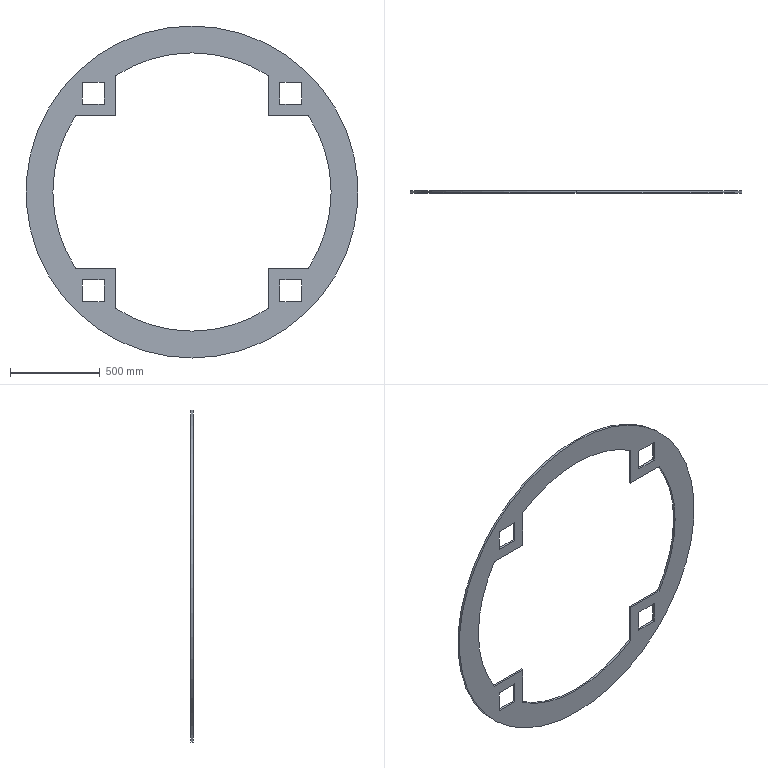Part | SolidWorks | features Extrusion 1 | 1 solid | 33 faces | box 1850 x 12 x 1850 mm | volume 10257241 mm3 | plane 26 | cylinder 7 | commonest cylinder face diameters 1550 x5 1850 x2
STEP:
#1=CARTESIAN_POINT('',(0.,12.,925.));
#2=VERTEX_POINT('',#1);
#3=CARTESIAN_POINT('',(0.,12.,-925.));
#4=VERTEX_POINT('',#3);
#5=CARTESIAN_POINT('',(0.,12.,0.));
#6=DIRECTION('',(0.,1.,0.));
#7=DIRECTION('',(0.,0.,1.));
#8=AXIS2_PLACEMENT_3D('',#5,#6,#7);
#9=CIRCLE('',#8,925.);
#10=EDGE_CURVE('',#2,#4,#9,.T.);
#11=ORIENTED_EDGE('',*,*,#10,.F.);
#12=CARTESIAN_POINT('',(0.,0.,925.));
#13=VERTEX_POINT('',#12);
#14=CARTESIAN_POINT('',(0.,12.,925.));
#15=DIRECTION('',(0.,-1.,0.));
#16=VECTOR('',#15,1000.);
#17=LINE('',#14,#16);
#18=EDGE_CURVE('',#2,#13,#17,.T.);
#19=ORIENTED_EDGE('',*,*,#18,.T.);
#20=CARTESIAN_POINT('',(0.,0.,-925.));
#21=VERTEX_POINT('',#20);
#22=CARTESIAN_POINT('',(0.,0.,0.));
#23=DIRECTION('',(0.,1.,0.));
#24=DIRECTION('',(0.,0.,1.));
#25=AXIS2_PLACEMENT_3D('',#22,#23,#24);
#26=CIRCLE('',#25,925.);
#27=EDGE_CURVE('',#13,#21,#26,.T.);
#28=ORIENTED_EDGE('',*,*,#27,.T.);
#29=CARTESIAN_POINT('',(0.,12.,-925.));
#30=DIRECTION('',(0.,-1.,0.));
#31=VECTOR('',#30,1000.);
#32=LINE('',#29,#31);
#33=EDGE_CURVE('',#4,#21,#32,.T.);
#34=ORIENTED_EDGE('',*,*,#33,.F.);
#35=EDGE_LOOP('',(#11,#19,#28,#34));
#36=FACE_OUTER_BOUND('',#35,.T.);
#37=CARTESIAN_POINT('',(0.,12.,0.));
#38=DIRECTION('',(0.,-1.,0.));
#39=DIRECTION('',(0.,0.,-1.));
#40=AXIS2_PLACEMENT_3D('',#37,#38,#39);
#41=CYLINDRICAL_SURFACE('',#40,925.);
#42=ADVANCED_FACE('',(#36),#41,.T.);
#43=CARTESIAN_POINT('',(425.,12.,-648.074));
#44=VERTEX_POINT('',#43);
#45=CARTESIAN_POINT('',(0.,12.,-775.));
#46=VERTEX_POINT('',#45);
#47=CARTESIAN_POINT('',(0.,12.,0.));
#48=DIRECTION('',(0.,1.,0.));
#49=DIRECTION('',(0.,0.,1.));
#50=AXIS2_PLACEMENT_3D('',#47,#48,#49);
#51=CIRCLE('',#50,775.);
#52=EDGE_CURVE('',#44,#46,#51,.T.);
#53=ORIENTED_EDGE('',*,*,#52,.T.);
#54=CARTESIAN_POINT('',(0.,0.,-775.));
#55=VERTEX_POINT('',#54);
#56=CARTESIAN_POINT('',(0.,12.,-775.));
#57=DIRECTION('',(0.,-1.,0.));
#58=VECTOR('',#57,1000.);
#59=LINE('',#56,#58);
#60=EDGE_CURVE('',#46,#55,#59,.T.);
#61=ORIENTED_EDGE('',*,*,#60,.T.);
#62=CARTESIAN_POINT('',(425.,0.,-648.074));
#63=VERTEX_POINT('',#62);
#64=CARTESIAN_POINT('',(0.,0.,0.));
#65=DIRECTION('',(0.,1.,0.));
#66=DIRECTION('',(0.,0.,1.));
#67=AXIS2_PLACEMENT_3D('',#64,#65,#66);
#68=CIRCLE('',#67,775.);
#69=EDGE_CURVE('',#63,#55,#68,.T.);
#70=ORIENTED_EDGE('',*,*,#69,.F.);
#71=CARTESIAN_POINT('',(425.,12.,-648.074));
#72=DIRECTION('',(0.,-1.,0.));
#73=VECTOR('',#72,1000.);
#74=LINE('',#71,#73);
#75=EDGE_CURVE('',#44,#63,#74,.T.);
#76=ORIENTED_EDGE('',*,*,#75,.F.);
#77=EDGE_LOOP('',(#53,#61,#70,#76));
#78=FACE_OUTER_BOUND('',#77,.T.);
#79=CARTESIAN_POINT('',(0.,12.,0.));
#80=DIRECTION('',(0.,-1.,0.));
#81=DIRECTION('',(0.,0.,-1.));
#82=AXIS2_PLACEMENT_3D('',#79,#80,#81);
#83=CYLINDRICAL_SURFACE('',#82,775.);
#84=ADVANCED_FACE('',(#78),#83,.F.);
#85=CARTESIAN_POINT('',(-489.,0.,-489.));
#86=VERTEX_POINT('',#85);
#87=CARTESIAN_POINT('',(-489.,0.,-611.));
#88=VERTEX_POINT('',#87);
#89=CARTESIAN_POINT('',(-489.,0.,0.));
#90=DIRECTION('',(0.,0.,-1.));
#91=VECTOR('',#90,1000.);
#92=LINE('',#89,#91);
#93=EDGE_CURVE('',#86,#88,#92,.T.);
#94=ORIENTED_EDGE('',*,*,#93,.F.);
#95=CARTESIAN_POINT('',(-489.,12.,-489.));
#96=VERTEX_POINT('',#95);
#97=CARTESIAN_POINT('',(-489.,12.,-489.));
#98=DIRECTION('',(0.,-1.,0.));
#99=VECTOR('',#98,1000.);
#100=LINE('',#97,#99);
#101=EDGE_CURVE('',#96,#86,#100,.T.);
#102=ORIENTED_EDGE('',*,*,#101,.F.);
#103=CARTESIAN_POINT('',(-489.,12.,-611.));
#104=VERTEX_POINT('',#103);
#105=CARTESIAN_POINT('',(-489.,12.,0.));
#106=DIRECTION('',(0.,0.,-1.));
#107=VECTOR('',#106,1000.);
#108=LINE('',#105,#107);
#109=EDGE_CURVE('',#96,#104,#108,.T.);
#110=ORIENTED_EDGE('',*,*,#109,.T.);
#111=CARTESIAN_POINT('',(-489.,12.,-611.));
#112=DIRECTION('',(0.,-1.,0.));
#113=VECTOR('',#112,1000.);
#114=LINE('',#111,#113);
#115=EDGE_CURVE('',#104,#88,#114,.T.);
#116=ORIENTED_EDGE('',*,*,#115,.T.);
#117=EDGE_LOOP('',(#94,#102,#110,#116));
#118=FACE_OUTER_BOUND('',#117,.T.);
#119=CARTESIAN_POINT('',(-489.,12.,0.));
#120=DIRECTION('',(-1.,0.,0.));
#121=DIRECTION('',(0.,0.,1.));
#122=AXIS2_PLACEMENT_3D('',#119,#120,#121);
#123=PLANE('',#122);
#124=ADVANCED_FACE('',(#118),#123,.T.);
#125=CARTESIAN_POINT('',(-611.,0.,-489.));
#126=VERTEX_POINT('',#125);
#127=CARTESIAN_POINT('',(0.,0.,-489.));
#128=DIRECTION('',(-1.,0.,0.));
#129=VECTOR('',#128,1000.);
#130=LINE('',#127,#129);
#131=EDGE_CURVE('',#86,#126,#130,.T.);
#132=ORIENTED_EDGE('',*,*,#131,.T.);
#133=CARTESIAN_POINT('',(-611.,12.,-489.));
#134=VERTEX_POINT('',#133);
#135=CARTESIAN_POINT('',(-611.,12.,-489.));
#136=DIRECTION('',(0.,-1.,0.));
#137=VECTOR('',#136,1000.);
#138=LINE('',#135,#137);
#139=EDGE_CURVE('',#134,#126,#138,.T.);
#140=ORIENTED_EDGE('',*,*,#139,.F.);
#141=CARTESIAN_POINT('',(0.,12.,-489.));
#142=DIRECTION('',(-1.,0.,0.));
#143=VECTOR('',#142,1000.);
#144=LINE('',#141,#143);
#145=EDGE_CURVE('',#96,#134,#144,.T.);
#146=ORIENTED_EDGE('',*,*,#145,.F.);
#147=ORIENTED_EDGE('',*,*,#101,.T.);
#148=EDGE_LOOP('',(#132,#140,#146,#147));
#149=FACE_OUTER_BOUND('',#148,.T.);
#150=CARTESIAN_POINT('',(0.,12.,-489.));
#151=DIRECTION('',(0.,0.,1.));
#152=DIRECTION('',(1.,0.,0.));
#153=AXIS2_PLACEMENT_3D('',#150,#151,#152);
#154=PLANE('',#153);
#155=ADVANCED_FACE('',(#149),#154,.F.);
#156=CARTESIAN_POINT('',(-611.,0.,-611.));
#157=VERTEX_POINT('',#156);
#158=CARTESIAN_POINT('',(-611.,0.,0.));
#159=DIRECTION('',(0.,0.,-1.));
#160=VECTOR('',#159,1000.);
#161=LINE('',#158,#160);
#162=EDGE_CURVE('',#126,#157,#161,.T.);
#163=ORIENTED_EDGE('',*,*,#162,.T.);
#164=CARTESIAN_POINT('',(-611.,12.,-611.));
#165=VERTEX_POINT('',#164);
#166=CARTESIAN_POINT('',(-611.,12.,-611.));
#167=DIRECTION('',(0.,-1.,0.));
#168=VECTOR('',#167,1000.);
#169=LINE('',#166,#168);
#170=EDGE_CURVE('',#165,#157,#169,.T.);
#171=ORIENTED_EDGE('',*,*,#170,.F.);
#172=CARTESIAN_POINT('',(-611.,12.,0.));
#173=DIRECTION('',(0.,0.,-1.));
#174=VECTOR('',#173,1000.);
#175=LINE('',#172,#174);
#176=EDGE_CURVE('',#134,#165,#175,.T.);
#177=ORIENTED_EDGE('',*,*,#176,.F.);
#178=ORIENTED_EDGE('',*,*,#139,.T.);
#179=EDGE_LOOP('',(#163,#171,#177,#178));
#180=FACE_OUTER_BOUND('',#179,.T.);
#181=CARTESIAN_POINT('',(-611.,12.,0.));
#182=DIRECTION('',(-1.,0.,0.));
#183=DIRECTION('',(0.,0.,1.));
#184=AXIS2_PLACEMENT_3D('',#181,#182,#183);
#185=PLANE('',#184);
#186=ADVANCED_FACE('',(#180),#185,.F.);
#187=CARTESIAN_POINT('',(-489.,0.,489.));
#188=VERTEX_POINT('',#187);
#189=CARTESIAN_POINT('',(-611.,0.,489.));
#190=VERTEX_POINT('',#189);
#191=CARTESIAN_POINT('',(0.,0.,489.));
#192=DIRECTION('',(-1.,0.,0.));
#193=VECTOR('',#192,1000.);
#194=LINE('',#191,#193);
#195=EDGE_CURVE('',#188,#190,#194,.T.);
#196=ORIENTED_EDGE('',*,*,#195,.F.);
#197=CARTESIAN_POINT('',(-489.,12.,489.));
#198=VERTEX_POINT('',#197);
#199=CARTESIAN_POINT('',(-489.,12.,489.));
#200=DIRECTION('',(0.,-1.,0.));
#201=VECTOR('',#200,1000.);
#202=LINE('',#199,#201);
#203=EDGE_CURVE('',#198,#188,#202,.T.);
#204=ORIENTED_EDGE('',*,*,#203,.F.);
#205=CARTESIAN_POINT('',(-611.,12.,489.));
#206=VERTEX_POINT('',#205);
#207=CARTESIAN_POINT('',(0.,12.,489.));
#208=DIRECTION('',(-1.,0.,0.));
#209=VECTOR('',#208,1000.);
#210=LINE('',#207,#209);
#211=EDGE_CURVE('',#198,#206,#210,.T.);
#212=ORIENTED_EDGE('',*,*,#211,.T.);
#213=CARTESIAN_POINT('',(-611.,12.,489.));
#214=DIRECTION('',(0.,-1.,0.));
#215=VECTOR('',#214,1000.);
#216=LINE('',#213,#215);
#217=EDGE_CURVE('',#206,#190,#216,.T.);
#218=ORIENTED_EDGE('',*,*,#217,.T.);
#219=EDGE_LOOP('',(#196,#204,#212,#218));
#220=FACE_OUTER_BOUND('',#219,.T.);
#221=CARTESIAN_POINT('',(0.,12.,489.));
#222=DIRECTION('',(0.,0.,1.));
#223=DIRECTION('',(1.,0.,0.));
#224=AXIS2_PLACEMENT_3D('',#221,#222,#223);
#225=PLANE('',#224);
#226=ADVANCED_FACE('',(#220),#225,.T.);
#227=CARTESIAN_POINT('',(-489.,0.,611.));
#228=VERTEX_POINT('',#227);
#229=CARTESIAN_POINT('',(-489.,0.,0.));
#230=DIRECTION('',(0.,0.,1.));
#231=VECTOR('',#230,1000.);
#232=LINE('',#229,#231);
#233=EDGE_CURVE('',#188,#228,#232,.T.);
#234=ORIENTED_EDGE('',*,*,#233,.T.);
#235=CARTESIAN_POINT('',(-489.,12.,611.));
#236=VERTEX_POINT('',#235);
#237=CARTESIAN_POINT('',(-489.,12.,611.));
#238=DIRECTION('',(0.,-1.,0.));
#239=VECTOR('',#238,1000.);
#240=LINE('',#237,#239);
#241=EDGE_CURVE('',#236,#228,#240,.T.);
#242=ORIENTED_EDGE('',*,*,#241,.F.);
#243=CARTESIAN_POINT('',(-489.,12.,0.));
#244=DIRECTION('',(0.,0.,1.));
#245=VECTOR('',#244,1000.);
#246=LINE('',#243,#245);
#247=EDGE_CURVE('',#198,#236,#246,.T.);
#248=ORIENTED_EDGE('',*,*,#247,.F.);
#249=ORIENTED_EDGE('',*,*,#203,.T.);
#250=EDGE_LOOP('',(#234,#242,#248,#249));
#251=FACE_OUTER_BOUND('',#250,.T.);
#252=CARTESIAN_POINT('',(-489.,12.,0.));
#253=DIRECTION('',(1.,0.,0.));
#254=DIRECTION('',(0.,0.,-1.));
#255=AXIS2_PLACEMENT_3D('',#252,#253,#254);
#256=PLANE('',#255);
#257=ADVANCED_FACE('',(#251),#256,.F.);
#258=CARTESIAN_POINT('',(-611.,0.,611.));
#259=VERTEX_POINT('',#258);
#260=CARTESIAN_POINT('',(0.,0.,611.));
#261=DIRECTION('',(-1.,0.,0.));
#262=VECTOR('',#261,1000.);
#263=LINE('',#260,#262);
#264=EDGE_CURVE('',#228,#259,#263,.T.);
#265=ORIENTED_EDGE('',*,*,#264,.T.);
#266=CARTESIAN_POINT('',(-611.,12.,611.));
#267=VERTEX_POINT('',#266);
#268=CARTESIAN_POINT('',(-611.,12.,611.));
#269=DIRECTION('',(0.,-1.,0.));
#270=VECTOR('',#269,1000.);
#271=LINE('',#268,#270);
#272=EDGE_CURVE('',#267,#259,#271,.T.);
#273=ORIENTED_EDGE('',*,*,#272,.F.);
#274=CARTESIAN_POINT('',(0.,12.,611.));
#275=DIRECTION('',(-1.,0.,0.));
#276=VECTOR('',#275,1000.);
#277=LINE('',#274,#276);
#278=EDGE_CURVE('',#236,#267,#277,.T.);
#279=ORIENTED_EDGE('',*,*,#278,.F.);
#280=ORIENTED_EDGE('',*,*,#241,.T.);
#281=EDGE_LOOP('',(#265,#273,#279,#280));
#282=FACE_OUTER_BOUND('',#281,.T.);
#283=CARTESIAN_POINT('',(0.,12.,611.));
#284=DIRECTION('',(0.,0.,1.));
#285=DIRECTION('',(1.,0.,0.));
#286=AXIS2_PLACEMENT_3D('',#283,#284,#285);
#287=PLANE('',#286);
#288=ADVANCED_FACE('',(#282),#287,.F.);
#289=CARTESIAN_POINT('',(489.,0.,489.));
#290=VERTEX_POINT('',#289);
#291=CARTESIAN_POINT('',(489.,0.,611.));
#292=VERTEX_POINT('',#291);
#293=CARTESIAN_POINT('',(489.,0.,0.));
#294=DIRECTION('',(0.,0.,1.));
#295=VECTOR('',#294,1000.);
#296=LINE('',#293,#295);
#297=EDGE_CURVE('',#290,#292,#296,.T.);
#298=ORIENTED_EDGE('',*,*,#297,.F.);
#299=CARTESIAN_POINT('',(489.,12.,489.));
#300=VERTEX_POINT('',#299);
#301=CARTESIAN_POINT('',(489.,12.,489.));
#302=DIRECTION('',(0.,-1.,0.));
#303=VECTOR('',#302,1000.);
#304=LINE('',#301,#303);
#305=EDGE_CURVE('',#300,#290,#304,.T.);
#306=ORIENTED_EDGE('',*,*,#305,.F.);
#307=CARTESIAN_POINT('',(489.,12.,611.));
#308=VERTEX_POINT('',#307);
#309=CARTESIAN_POINT('',(489.,12.,0.));
#310=DIRECTION('',(0.,0.,1.));
#311=VECTOR('',#310,1000.);
#312=LINE('',#309,#311);
#313=EDGE_CURVE('',#300,#308,#312,.T.);
#314=ORIENTED_EDGE('',*,*,#313,.T.);
#315=CARTESIAN_POINT('',(489.,12.,611.));
#316=DIRECTION('',(0.,-1.,0.));
#317=VECTOR('',#316,1000.);
#318=LINE('',#315,#317);
#319=EDGE_CURVE('',#308,#292,#318,.T.);
#320=ORIENTED_EDGE('',*,*,#319,.T.);
#321=EDGE_LOOP('',(#298,#306,#314,#320));
#322=FACE_OUTER_BOUND('',#321,.T.);
#323=CARTESIAN_POINT('',(489.,12.,0.));
#324=DIRECTION('',(1.,0.,0.));
#325=DIRECTION('',(0.,0.,-1.));
#326=AXIS2_PLACEMENT_3D('',#323,#324,#325);
#327=PLANE('',#326);
#328=ADVANCED_FACE('',(#322),#327,.T.);
#329=CARTESIAN_POINT('',(611.,0.,489.));
#330=VERTEX_POINT('',#329);
#331=CARTESIAN_POINT('',(0.,0.,489.));
#332=DIRECTION('',(1.,0.,0.));
#333=VECTOR('',#332,1000.);
#334=LINE('',#331,#333);
#335=EDGE_CURVE('',#290,#330,#334,.T.);
#336=ORIENTED_EDGE('',*,*,#335,.T.);
#337=CARTESIAN_POINT('',(611.,12.,489.));
#338=VERTEX_POINT('',#337);
#339=CARTESIAN_POINT('',(611.,12.,489.));
#340=DIRECTION('',(0.,-1.,0.));
#341=VECTOR('',#340,1000.);
#342=LINE('',#339,#341);
#343=EDGE_CURVE('',#338,#330,#342,.T.);
#344=ORIENTED_EDGE('',*,*,#343,.F.);
#345=CARTESIAN_POINT('',(0.,12.,489.));
#346=DIRECTION('',(1.,0.,0.));
#347=VECTOR('',#346,1000.);
#348=LINE('',#345,#347);
#349=EDGE_CURVE('',#300,#338,#348,.T.);
#350=ORIENTED_EDGE('',*,*,#349,.F.);
#351=ORIENTED_EDGE('',*,*,#305,.T.);
#352=EDGE_LOOP('',(#336,#344,#350,#351));
#353=FACE_OUTER_BOUND('',#352,.T.);
#354=CARTESIAN_POINT('',(0.,12.,489.));
#355=DIRECTION('',(0.,0.,-1.));
#356=DIRECTION('',(-1.,0.,0.));
#357=AXIS2_PLACEMENT_3D('',#354,#355,#356);
#358=PLANE('',#357);
#359=ADVANCED_FACE('',(#353),#358,.F.);
#360=CARTESIAN_POINT('',(611.,0.,611.));
#361=VERTEX_POINT('',#360);
#362=CARTESIAN_POINT('',(611.,0.,0.));
#363=DIRECTION('',(0.,0.,1.));
#364=VECTOR('',#363,1000.);
#365=LINE('',#362,#364);
#366=EDGE_CURVE('',#330,#361,#365,.T.);
#367=ORIENTED_EDGE('',*,*,#366,.T.);
#368=CARTESIAN_POINT('',(611.,12.,611.));
#369=VERTEX_POINT('',#368);
#370=CARTESIAN_POINT('',(611.,12.,611.));
#371=DIRECTION('',(0.,-1.,0.));
#372=VECTOR('',#371,1000.);
#373=LINE('',#370,#372);
#374=EDGE_CURVE('',#369,#361,#373,.T.);
#375=ORIENTED_EDGE('',*,*,#374,.F.);
#376=CARTESIAN_POINT('',(611.,12.,0.));
#377=DIRECTION('',(0.,0.,1.));
#378=VECTOR('',#377,1000.);
#379=LINE('',#376,#378);
#380=EDGE_CURVE('',#338,#369,#379,.T.);
#381=ORIENTED_EDGE('',*,*,#380,.F.);
#382=ORIENTED_EDGE('',*,*,#343,.T.);
#383=EDGE_LOOP('',(#367,#375,#381,#382));
#384=FACE_OUTER_BOUND('',#383,.T.);
#385=CARTESIAN_POINT('',(611.,12.,0.));
#386=DIRECTION('',(1.,0.,0.));
#387=DIRECTION('',(0.,0.,-1.));
#388=AXIS2_PLACEMENT_3D('',#385,#386,#387);
#389=PLANE('',#388);
#390=ADVANCED_FACE('',(#384),#389,.F.);
#391=CARTESIAN_POINT('',(489.,0.,-489.));
#392=VERTEX_POINT('',#391);
#393=CARTESIAN_POINT('',(611.,0.,-489.));
#394=VERTEX_POINT('',#393);
#395=CARTESIAN_POINT('',(0.,0.,-489.));
#396=DIRECTION('',(1.,0.,0.));
#397=VECTOR('',#396,1000.);
#398=LINE('',#395,#397);
#399=EDGE_CURVE('',#392,#394,#398,.T.);
#400=ORIENTED_EDGE('',*,*,#399,.F.);
#401=CARTESIAN_POINT('',(489.,12.,-489.));
#402=VERTEX_POINT('',#401);
#403=CARTESIAN_POINT('',(489.,12.,-489.));
#404=DIRECTION('',(0.,-1.,0.));
#405=VECTOR('',#404,1000.);
#406=LINE('',#403,#405);
#407=EDGE_CURVE('',#402,#392,#406,.T.);
#408=ORIENTED_EDGE('',*,*,#407,.F.);
#409=CARTESIAN_POINT('',(611.,12.,-489.));
#410=VERTEX_POINT('',#409);
#411=CARTESIAN_POINT('',(0.,12.,-489.));
#412=DIRECTION('',(1.,0.,0.));
#413=VECTOR('',#412,1000.);
#414=LINE('',#411,#413);
#415=EDGE_CURVE('',#402,#410,#414,.T.);
#416=ORIENTED_EDGE('',*,*,#415,.T.);
#417=CARTESIAN_POINT('',(611.,12.,-489.));
#418=DIRECTION('',(0.,-1.,0.));
#419=VECTOR('',#418,1000.);
#420=LINE('',#417,#419);
#421=EDGE_CURVE('',#410,#394,#420,.T.);
#422=ORIENTED_EDGE('',*,*,#421,.T.);
#423=EDGE_LOOP('',(#400,#408,#416,#422));
#424=FACE_OUTER_BOUND('',#423,.T.);
#425=CARTESIAN_POINT('',(0.,12.,-489.));
#426=DIRECTION('',(0.,0.,-1.));
#427=DIRECTION('',(-1.,0.,0.));
#428=AXIS2_PLACEMENT_3D('',#425,#426,#427);
#429=PLANE('',#428);
#430=ADVANCED_FACE('',(#424),#429,.T.);
#431=CARTESIAN_POINT('',(489.,0.,-611.));
#432=VERTEX_POINT('',#431);
#433=CARTESIAN_POINT('',(489.,0.,0.));
#434=DIRECTION('',(0.,0.,-1.));
#435=VECTOR('',#434,1000.);
#436=LINE('',#433,#435);
#437=EDGE_CURVE('',#392,#432,#436,.T.);
#438=ORIENTED_EDGE('',*,*,#437,.T.);
#439=CARTESIAN_POINT('',(489.,12.,-611.));
#440=VERTEX_POINT('',#439);
#441=CARTESIAN_POINT('',(489.,12.,-611.));
#442=DIRECTION('',(0.,-1.,0.));
#443=VECTOR('',#442,1000.);
#444=LINE('',#441,#443);
#445=EDGE_CURVE('',#440,#432,#444,.T.);
#446=ORIENTED_EDGE('',*,*,#445,.F.);
#447=CARTESIAN_POINT('',(489.,12.,0.));
#448=DIRECTION('',(0.,0.,-1.));
#449=VECTOR('',#448,1000.);
#450=LINE('',#447,#449);
#451=EDGE_CURVE('',#402,#440,#450,.T.);
#452=ORIENTED_EDGE('',*,*,#451,.F.);
#453=ORIENTED_EDGE('',*,*,#407,.T.);
#454=EDGE_LOOP('',(#438,#446,#452,#453));
#455=FACE_OUTER_BOUND('',#454,.T.);
#456=CARTESIAN_POINT('',(489.,12.,0.));
#457=DIRECTION('',(-1.,0.,0.));
#458=DIRECTION('',(0.,0.,1.));
#459=AXIS2_PLACEMENT_3D('',#456,#457,#458);
#460=PLANE('',#459);
#461=ADVANCED_FACE('',(#455),#460,.F.);
#462=CARTESIAN_POINT('',(611.,0.,-611.));
#463=VERTEX_POINT('',#462);
#464=CARTESIAN_POINT('',(0.,0.,-611.));
#465=DIRECTION('',(1.,0.,0.));
#466=VECTOR('',#465,1000.);
#467=LINE('',#464,#466);
#468=EDGE_CURVE('',#432,#463,#467,.T.);
#469=ORIENTED_EDGE('',*,*,#468,.T.);
#470=CARTESIAN_POINT('',(611.,12.,-611.));
#471=VERTEX_POINT('',#470);
#472=CARTESIAN_POINT('',(611.,12.,-611.));
#473=DIRECTION('',(0.,-1.,0.));
#474=VECTOR('',#473,1000.);
#475=LINE('',#472,#474);
#476=EDGE_CURVE('',#471,#463,#475,.T.);
#477=ORIENTED_EDGE('',*,*,#476,.F.);
#478=CARTESIAN_POINT('',(0.,12.,-611.));
#479=DIRECTION('',(1.,0.,0.));
#480=VECTOR('',#479,1000.);
#481=LINE('',#478,#480);
#482=EDGE_CURVE('',#440,#471,#481,.T.);
#483=ORIENTED_EDGE('',*,*,#482,.F.);
#484=ORIENTED_EDGE('',*,*,#445,.T.);
#485=EDGE_LOOP('',(#469,#477,#483,#484));
#486=FACE_OUTER_BOUND('',#485,.T.);
#487=CARTESIAN_POINT('',(0.,12.,-611.));
#488=DIRECTION('',(0.,0.,-1.));
#489=DIRECTION('',(-1.,0.,0.));
#490=AXIS2_PLACEMENT_3D('',#487,#488,#489);
#491=PLANE('',#490);
#492=ADVANCED_FACE('',(#486),#491,.F.);
#493=CARTESIAN_POINT('',(648.074,0.,425.));
#494=VERTEX_POINT('',#493);
#495=CARTESIAN_POINT('',(648.074,0.,-425.));
#496=VERTEX_POINT('',#495);
#497=CARTESIAN_POINT('',(0.,0.,0.));
#498=DIRECTION('',(0.,1.,0.));
#499=DIRECTION('',(0.,0.,1.));
#500=AXIS2_PLACEMENT_3D('',#497,#498,#499);
#501=CIRCLE('',#500,775.);
#502=EDGE_CURVE('',#494,#496,#501,.T.);
#503=ORIENTED_EDGE('',*,*,#502,.F.);
#504=CARTESIAN_POINT('',(648.074,12.,425.));
#505=VERTEX_POINT('',#504);
#506=CARTESIAN_POINT('',(648.074,12.,425.));
#507=DIRECTION('',(0.,-1.,0.));
#508=VECTOR('',#507,1000.);
#509=LINE('',#506,#508);
#510=EDGE_CURVE('',#505,#494,#509,.T.);
#511=ORIENTED_EDGE('',*,*,#510,.F.);
#512=CARTESIAN_POINT('',(648.074,12.,-425.));
#513=VERTEX_POINT('',#512);
#514=CARTESIAN_POINT('',(0.,12.,0.));
#515=DIRECTION('',(0.,1.,0.));
#516=DIRECTION('',(0.,0.,1.));
#517=AXIS2_PLACEMENT_3D('',#514,#515,#516);
#518=CIRCLE('',#517,775.);
#519=EDGE_CURVE('',#505,#513,#518,.T.);
#520=ORIENTED_EDGE('',*,*,#519,.T.);
#521=CARTESIAN_POINT('',(648.074,12.,-425.));
#522=DIRECTION('',(0.,-1.,0.));
#523=VECTOR('',#522,1000.);
#524=LINE('',#521,#523);
#525=EDGE_CURVE('',#513,#496,#524,.T.);
#526=ORIENTED_EDGE('',*,*,#525,.T.);
#527=EDGE_LOOP('',(#503,#511,#520,#526));
#528=FACE_OUTER_BOUND('',#527,.T.);
#529=CARTESIAN_POINT('',(0.,12.,0.));
#530=DIRECTION('',(0.,-1.,0.));
#531=DIRECTION('',(0.,0.,-1.));
#532=AXIS2_PLACEMENT_3D('',#529,#530,#531);
#533=CYLINDRICAL_SURFACE('',#532,775.);
#534=ADVANCED_FACE('',(#528),#533,.F.);
#535=CARTESIAN_POINT('',(425.,0.,425.));
#536=VERTEX_POINT('',#535);
#537=CARTESIAN_POINT('',(0.,0.,425.));
#538=DIRECTION('',(1.,0.,0.));
#539=VECTOR('',#538,1000.);
#540=LINE('',#537,#539);
#541=EDGE_CURVE('',#536,#494,#540,.T.);
#542=ORIENTED_EDGE('',*,*,#541,.F.);
#543=CARTESIAN_POINT('',(425.,12.,425.));
#544=VERTEX_POINT('',#543);
#545=CARTESIAN_POINT('',(425.,12.,425.));
#546=DIRECTION('',(0.,-1.,0.));
#547=VECTOR('',#546,1000.);
#548=LINE('',#545,#547);
#549=EDGE_CURVE('',#544,#536,#548,.T.);
#550=ORIENTED_EDGE('',*,*,#549,.F.);
#551=CARTESIAN_POINT('',(0.,12.,425.));
#552=DIRECTION('',(1.,0.,0.));
#553=VECTOR('',#552,1000.);
#554=LINE('',#551,#553);
#555=EDGE_CURVE('',#544,#505,#554,.T.);
#556=ORIENTED_EDGE('',*,*,#555,.T.);
#557=ORIENTED_EDGE('',*,*,#510,.T.);
#558=EDGE_LOOP('',(#542,#550,#556,#557));
#559=FACE_OUTER_BOUND('',#558,.T.);
#560=CARTESIAN_POINT('',(0.,12.,425.));
#561=DIRECTION('',(0.,0.,-1.));
#562=DIRECTION('',(-1.,0.,0.));
#563=AXIS2_PLACEMENT_3D('',#560,#561,#562);
#564=PLANE('',#563);
#565=ADVANCED_FACE('',(#559),#564,.T.);
#566=CARTESIAN_POINT('',(425.,0.,648.074));
#567=VERTEX_POINT('',#566);
#568=CARTESIAN_POINT('',(425.,0.,0.));
#569=DIRECTION('',(0.,0.,1.));
#570=VECTOR('',#569,1000.);
#571=LINE('',#568,#570);
#572=EDGE_CURVE('',#536,#567,#571,.T.);
#573=ORIENTED_EDGE('',*,*,#572,.T.);
#574=CARTESIAN_POINT('',(425.,12.,648.074));
#575=VERTEX_POINT('',#574);
#576=CARTESIAN_POINT('',(425.,12.,648.074));
#577=DIRECTION('',(0.,-1.,0.));
#578=VECTOR('',#577,1000.);
#579=LINE('',#576,#578);
#580=EDGE_CURVE('',#575,#567,#579,.T.);
#581=ORIENTED_EDGE('',*,*,#580,.F.);
#582=CARTESIAN_POINT('',(425.,12.,0.));
#583=DIRECTION('',(0.,0.,1.));
#584=VECTOR('',#583,1000.);
#585=LINE('',#582,#584);
#586=EDGE_CURVE('',#544,#575,#585,.T.);
#587=ORIENTED_EDGE('',*,*,#586,.F.);
#588=ORIENTED_EDGE('',*,*,#549,.T.);
#589=EDGE_LOOP('',(#573,#581,#587,#588));
#590=FACE_OUTER_BOUND('',#589,.T.);
#591=CARTESIAN_POINT('',(425.,12.,0.));
#592=DIRECTION('',(1.,0.,0.));
#593=DIRECTION('',(0.,0.,-1.));
#594=AXIS2_PLACEMENT_3D('',#591,#592,#593);
#595=PLANE('',#594);
#596=ADVANCED_FACE('',(#590),#595,.F.);
#597=CARTESIAN_POINT('',(-425.,0.,648.074));
#598=VERTEX_POINT('',#597);
#599=CARTESIAN_POINT('',(0.,0.,0.));
#600=DIRECTION('',(0.,1.,0.));
#601=DIRECTION('',(0.,0.,1.));
#602=AXIS2_PLACEMENT_3D('',#599,#600,#601);
#603=CIRCLE('',#602,775.);
#604=EDGE_CURVE('',#598,#567,#603,.T.);
#605=ORIENTED_EDGE('',*,*,#604,.F.);
#606=CARTESIAN_POINT('',(-425.,12.,648.074));
#607=VERTEX_POINT('',#606);
#608=CARTESIAN_POINT('',(-425.,12.,648.074));
#609=DIRECTION('',(0.,-1.,0.));
#610=VECTOR('',#609,1000.);
#611=LINE('',#608,#610);
#612=EDGE_CURVE('',#607,#598,#611,.T.);
#613=ORIENTED_EDGE('',*,*,#612,.F.);
#614=CARTESIAN_POINT('',(0.,12.,0.));
#615=DIRECTION('',(0.,1.,0.));
#616=DIRECTION('',(0.,0.,1.));
#617=AXIS2_PLACEMENT_3D('',#614,#615,#616);
#618=CIRCLE('',#617,775.);
#619=EDGE_CURVE('',#607,#575,#618,.T.);
#620=ORIENTED_EDGE('',*,*,#619,.T.);
#621=ORIENTED_EDGE('',*,*,#580,.T.);
#622=EDGE_LOOP('',(#605,#613,#620,#621));
#623=FACE_OUTER_BOUND('',#622,.T.);
#624=CARTESIAN_POINT('',(0.,12.,0.));
#625=DIRECTION('',(0.,-1.,0.));
#626=DIRECTION('',(0.,0.,-1.));
#627=AXIS2_PLACEMENT_3D('',#624,#625,#626);
#628=CYLINDRICAL_SURFACE('',#627,775.);
#629=ADVANCED_FACE('',(#623),#628,.F.);
#630=CARTESIAN_POINT('',(-425.,0.,425.));
#631=VERTEX_POINT('',#630);
#632=CARTESIAN_POINT('',(-425.,0.,0.));
#633=DIRECTION('',(0.,0.,1.));
#634=VECTOR('',#633,1000.);
#635=LINE('',#632,#634);
#636=EDGE_CURVE('',#631,#598,#635,.T.);
#637=ORIENTED_EDGE('',*,*,#636,.F.);
#638=CARTESIAN_POINT('',(-425.,12.,425.));
#639=VERTEX_POINT('',#638);
#640=CARTESIAN_POINT('',(-425.,12.,425.));
#641=DIRECTION('',(0.,-1.,0.));
#642=VECTOR('',#641,1000.);
#643=LINE('',#640,#642);
#644=EDGE_CURVE('',#639,#631,#643,.T.);
#645=ORIENTED_EDGE('',*,*,#644,.F.);
#646=CARTESIAN_POINT('',(-425.,12.,0.));
#647=DIRECTION('',(0.,0.,1.));
#648=VECTOR('',#647,1000.);
#649=LINE('',#646,#648);
#650=EDGE_CURVE('',#639,#607,#649,.T.);
#651=ORIENTED_EDGE('',*,*,#650,.T.);
#652=ORIENTED_EDGE('',*,*,#612,.T.);
#653=EDGE_LOOP('',(#637,#645,#651,#652));
#654=FACE_OUTER_BOUND('',#653,.T.);
#655=CARTESIAN_POINT('',(-425.,12.,0.));
#656=DIRECTION('',(1.,0.,0.));
#657=DIRECTION('',(0.,0.,-1.));
#658=AXIS2_PLACEMENT_3D('',#655,#656,#657);
#659=PLANE('',#658);
#660=ADVANCED_FACE('',(#654),#659,.T.);
#661=CARTESIAN_POINT('',(-648.074,0.,425.));
#662=VERTEX_POINT('',#661);
#663=CARTESIAN_POINT('',(0.,0.,425.));
#664=DIRECTION('',(-1.,0.,0.));
#665=VECTOR('',#664,1000.);
#666=LINE('',#663,#665);
#667=EDGE_CURVE('',#631,#662,#666,.T.);
#668=ORIENTED_EDGE('',*,*,#667,.T.);
#669=CARTESIAN_POINT('',(-648.074,12.,425.));
#670=VERTEX_POINT('',#669);
#671=CARTESIAN_POINT('',(-648.074,12.,425.));
#672=DIRECTION('',(0.,-1.,0.));
#673=VECTOR('',#672,1000.);
#674=LINE('',#671,#673);
#675=EDGE_CURVE('',#670,#662,#674,.T.);
#676=ORIENTED_EDGE('',*,*,#675,.F.);
#677=CARTESIAN_POINT('',(0.,12.,425.));
#678=DIRECTION('',(-1.,0.,0.));
#679=VECTOR('',#678,1000.);
#680=LINE('',#677,#679);
#681=EDGE_CURVE('',#639,#670,#680,.T.);
#682=ORIENTED_EDGE('',*,*,#681,.F.);
#683=ORIENTED_EDGE('',*,*,#644,.T.);
#684=EDGE_LOOP('',(#668,#676,#682,#683));
#685=FACE_OUTER_BOUND('',#684,.T.);
#686=CARTESIAN_POINT('',(0.,12.,425.));
#687=DIRECTION('',(0.,0.,1.));
#688=DIRECTION('',(1.,0.,0.));
#689=AXIS2_PLACEMENT_3D('',#686,#687,#688);
#690=PLANE('',#689);
#691=ADVANCED_FACE('',(#685),#690,.F.);
#692=CARTESIAN_POINT('',(-648.074,0.,-425.));
#693=VERTEX_POINT('',#692);
#694=CARTESIAN_POINT('',(0.,0.,0.));
#695=DIRECTION('',(0.,1.,0.));
#696=DIRECTION('',(0.,0.,1.));
#697=AXIS2_PLACEMENT_3D('',#694,#695,#696);
#698=CIRCLE('',#697,775.);
#699=EDGE_CURVE('',#693,#662,#698,.T.);
#700=ORIENTED_EDGE('',*,*,#699,.F.);
#701=CARTESIAN_POINT('',(-648.074,12.,-425.));
#702=VERTEX_POINT('',#701);
#703=CARTESIAN_POINT('',(-648.074,12.,-425.));
#704=DIRECTION('',(0.,-1.,0.));
#705=VECTOR('',#704,1000.);
#706=LINE('',#703,#705);
#707=EDGE_CURVE('',#702,#693,#706,.T.);
#708=ORIENTED_EDGE('',*,*,#707,.F.);
#709=CARTESIAN_POINT('',(0.,12.,0.));
#710=DIRECTION('',(0.,1.,0.));
#711=DIRECTION('',(0.,0.,1.));
#712=AXIS2_PLACEMENT_3D('',#709,#710,#711);
#713=CIRCLE('',#712,775.);
#714=EDGE_CURVE('',#702,#670,#713,.T.);
#715=ORIENTED_EDGE('',*,*,#714,.T.);
#716=ORIENTED_EDGE('',*,*,#675,.T.);
#717=EDGE_LOOP('',(#700,#708,#715,#716));
#718=FACE_OUTER_BOUND('',#717,.T.);
#719=CARTESIAN_POINT('',(0.,12.,0.));
#720=DIRECTION('',(0.,-1.,0.));
#721=DIRECTION('',(0.,0.,-1.));
#722=AXIS2_PLACEMENT_3D('',#719,#720,#721);
#723=CYLINDRICAL_SURFACE('',#722,775.);
#724=ADVANCED_FACE('',(#718),#723,.F.);
#725=CARTESIAN_POINT('',(-425.,0.,-425.));
#726=VERTEX_POINT('',#725);
#727=CARTESIAN_POINT('',(0.,0.,-425.));
#728=DIRECTION('',(-1.,0.,0.));
#729=VECTOR('',#728,1000.);
#730=LINE('',#727,#729);
#731=EDGE_CURVE('',#726,#693,#730,.T.);
#732=ORIENTED_EDGE('',*,*,#731,.F.);
#733=CARTESIAN_POINT('',(-425.,12.,-425.));
#734=VERTEX_POINT('',#733);
#735=CARTESIAN_POINT('',(-425.,12.,-425.));
#736=DIRECTION('',(0.,-1.,0.));
#737=VECTOR('',#736,1000.);
#738=LINE('',#735,#737);
#739=EDGE_CURVE('',#734,#726,#738,.T.);
#740=ORIENTED_EDGE('',*,*,#739,.F.);
#741=CARTESIAN_POINT('',(0.,12.,-425.));
#742=DIRECTION('',(-1.,0.,0.));
#743=VECTOR('',#742,1000.);
#744=LINE('',#741,#743);
#745=EDGE_CURVE('',#734,#702,#744,.T.);
#746=ORIENTED_EDGE('',*,*,#745,.T.);
#747=ORIENTED_EDGE('',*,*,#707,.T.);
#748=EDGE_LOOP('',(#732,#740,#746,#747));
#749=FACE_OUTER_BOUND('',#748,.T.);
#750=CARTESIAN_POINT('',(0.,12.,-425.));
#751=DIRECTION('',(0.,0.,1.));
#752=DIRECTION('',(1.,0.,0.));
#753=AXIS2_PLACEMENT_3D('',#750,#751,#752);
#754=PLANE('',#753);
#755=ADVANCED_FACE('',(#749),#754,.T.);
#756=CARTESIAN_POINT('',(-425.,0.,-648.074));
#757=VERTEX_POINT('',#756);
#758=CARTESIAN_POINT('',(-425.,0.,0.));
#759=DIRECTION('',(0.,0.,-1.));
#760=VECTOR('',#759,1000.);
#761=LINE('',#758,#760);
#762=EDGE_CURVE('',#726,#757,#761,.T.);
#763=ORIENTED_EDGE('',*,*,#762,.T.);
#764=CARTESIAN_POINT('',(-425.,12.,-648.074));
#765=VERTEX_POINT('',#764);
#766=CARTESIAN_POINT('',(-425.,12.,-648.074));
#767=DIRECTION('',(0.,-1.,0.));
#768=VECTOR('',#767,1000.);
#769=LINE('',#766,#768);
#770=EDGE_CURVE('',#765,#757,#769,.T.);
#771=ORIENTED_EDGE('',*,*,#770,.F.);
#772=CARTESIAN_POINT('',(-425.,12.,0.));
#773=DIRECTION('',(0.,0.,-1.));
#774=VECTOR('',#773,1000.);
#775=LINE('',#772,#774);
#776=EDGE_CURVE('',#734,#765,#775,.T.);
#777=ORIENTED_EDGE('',*,*,#776,.F.);
#778=ORIENTED_EDGE('',*,*,#739,.T.);
#779=EDGE_LOOP('',(#763,#771,#777,#778));
#780=FACE_OUTER_BOUND('',#779,.T.);
#781=CARTESIAN_POINT('',(-425.,12.,0.));
#782=DIRECTION('',(-1.,0.,0.));
#783=DIRECTION('',(0.,0.,1.));
#784=AXIS2_PLACEMENT_3D('',#781,#782,#783);
#785=PLANE('',#784);
#786=ADVANCED_FACE('',(#780),#785,.F.);
#787=ORIENTED_EDGE('',*,*,#60,.F.);
#788=CARTESIAN_POINT('',(0.,12.,0.));
#789=DIRECTION('',(0.,1.,0.));
#790=DIRECTION('',(0.,0.,1.));
#791=AXIS2_PLACEMENT_3D('',#788,#789,#790);
#792=CIRCLE('',#791,775.);
#793=EDGE_CURVE('',#46,#765,#792,.T.);
#794=ORIENTED_EDGE('',*,*,#793,.T.);
#795=ORIENTED_EDGE('',*,*,#770,.T.);
#796=CARTESIAN_POINT('',(0.,0.,0.));
#797=DIRECTION('',(0.,1.,0.));
#798=DIRECTION('',(0.,0.,1.));
#799=AXIS2_PLACEMENT_3D('',#796,#797,#798);
#800=CIRCLE('',#799,775.);
#801=EDGE_CURVE('',#55,#757,#800,.T.);
#802=ORIENTED_EDGE('',*,*,#801,.F.);
#803=EDGE_LOOP('',(#787,#794,#795,#802));
#804=FACE_OUTER_BOUND('',#803,.T.);
#805=CARTESIAN_POINT('',(0.,12.,0.));
#806=DIRECTION('',(0.,-1.,0.));
#807=DIRECTION('',(0.,0.,-1.));
#808=AXIS2_PLACEMENT_3D('',#805,#806,#807);
#809=CYLINDRICAL_SURFACE('',#808,775.);
#810=ADVANCED_FACE('',(#804),#809,.F.);
#811=CARTESIAN_POINT('',(425.,0.,-425.));
#812=VERTEX_POINT('',#811);
#813=CARTESIAN_POINT('',(425.,0.,0.));
#814=DIRECTION('',(0.,0.,-1.));
#815=VECTOR('',#814,1000.);
#816=LINE('',#813,#815);
#817=EDGE_CURVE('',#812,#63,#816,.T.);
#818=ORIENTED_EDGE('',*,*,#817,.F.);
#819=CARTESIAN_POINT('',(425.,12.,-425.));
#820=VERTEX_POINT('',#819);
#821=CARTESIAN_POINT('',(425.,12.,-425.));
#822=DIRECTION('',(0.,-1.,0.));
#823=VECTOR('',#822,1000.);
#824=LINE('',#821,#823);
#825=EDGE_CURVE('',#820,#812,#824,.T.);
#826=ORIENTED_EDGE('',*,*,#825,.F.);
#827=CARTESIAN_POINT('',(425.,12.,0.));
#828=DIRECTION('',(0.,0.,-1.));
#829=VECTOR('',#828,1000.);
#830=LINE('',#827,#829);
#831=EDGE_CURVE('',#820,#44,#830,.T.);
#832=ORIENTED_EDGE('',*,*,#831,.T.);
#833=ORIENTED_EDGE('',*,*,#75,.T.);
#834=EDGE_LOOP('',(#818,#826,#832,#833));
#835=FACE_OUTER_BOUND('',#834,.T.);
#836=CARTESIAN_POINT('',(425.,12.,0.));
#837=DIRECTION('',(-1.,0.,0.));
#838=DIRECTION('',(0.,0.,1.));
#839=AXIS2_PLACEMENT_3D('',#836,#837,#838);
#840=PLANE('',#839);
#841=ADVANCED_FACE('',(#835),#840,.T.);
#842=CARTESIAN_POINT('',(0.,0.,-611.));
#843=DIRECTION('',(-1.,0.,0.));
#844=VECTOR('',#843,1000.);
#845=LINE('',#842,#844);
#846=EDGE_CURVE('',#88,#157,#845,.T.);
#847=ORIENTED_EDGE('',*,*,#846,.F.);
#848=ORIENTED_EDGE('',*,*,#115,.F.);
#849=CARTESIAN_POINT('',(0.,12.,-611.));
#850=DIRECTION('',(-1.,0.,0.));
#851=VECTOR('',#850,1000.);
#852=LINE('',#849,#851);
#853=EDGE_CURVE('',#104,#165,#852,.T.);
#854=ORIENTED_EDGE('',*,*,#853,.T.);
#855=ORIENTED_EDGE('',*,*,#170,.T.);
#856=EDGE_LOOP('',(#847,#848,#854,#855));
#857=FACE_OUTER_BOUND('',#856,.T.);
#858=CARTESIAN_POINT('',(0.,12.,-611.));
#859=DIRECTION('',(0.,0.,1.));
#860=DIRECTION('',(1.,0.,0.));
#861=AXIS2_PLACEMENT_3D('',#858,#859,#860);
#862=PLANE('',#861);
#863=ADVANCED_FACE('',(#857),#862,.T.);
#864=CARTESIAN_POINT('',(-611.,0.,0.));
#865=DIRECTION('',(0.,0.,1.));
#866=VECTOR('',#865,1000.);
#867=LINE('',#864,#866);
#868=EDGE_CURVE('',#190,#259,#867,.T.);
#869=ORIENTED_EDGE('',*,*,#868,.F.);
#870=ORIENTED_EDGE('',*,*,#217,.F.);
#871=CARTESIAN_POINT('',(-611.,12.,0.));
#872=DIRECTION('',(0.,0.,1.));
#873=VECTOR('',#872,1000.);
#874=LINE('',#871,#873);
#875=EDGE_CURVE('',#206,#267,#874,.T.);
#876=ORIENTED_EDGE('',*,*,#875,.T.);
#877=ORIENTED_EDGE('',*,*,#272,.T.);
#878=EDGE_LOOP('',(#869,#870,#876,#877));
#879=FACE_OUTER_BOUND('',#878,.T.);
#880=CARTESIAN_POINT('',(-611.,12.,0.));
#881=DIRECTION('',(1.,0.,0.));
#882=DIRECTION('',(0.,0.,-1.));
#883=AXIS2_PLACEMENT_3D('',#880,#881,#882);
#884=PLANE('',#883);
#885=ADVANCED_FACE('',(#879),#884,.T.);
#886=CARTESIAN_POINT('',(0.,0.,611.));
#887=DIRECTION('',(1.,0.,0.));
#888=VECTOR('',#887,1000.);
#889=LINE('',#886,#888);
#890=EDGE_CURVE('',#292,#361,#889,.T.);
#891=ORIENTED_EDGE('',*,*,#890,.F.);
#892=ORIENTED_EDGE('',*,*,#319,.F.);
#893=CARTESIAN_POINT('',(0.,12.,611.));
#894=DIRECTION('',(1.,0.,0.));
#895=VECTOR('',#894,1000.);
#896=LINE('',#893,#895);
#897=EDGE_CURVE('',#308,#369,#896,.T.);
#898=ORIENTED_EDGE('',*,*,#897,.T.);
#899=ORIENTED_EDGE('',*,*,#374,.T.);
#900=EDGE_LOOP('',(#891,#892,#898,#899));
#901=FACE_OUTER_BOUND('',#900,.T.);
#902=CARTESIAN_POINT('',(0.,12.,611.));
#903=DIRECTION('',(0.,0.,-1.));
#904=DIRECTION('',(-1.,0.,0.));
#905=AXIS2_PLACEMENT_3D('',#902,#903,#904);
#906=PLANE('',#905);
#907=ADVANCED_FACE('',(#901),#906,.T.);
#908=CARTESIAN_POINT('',(611.,0.,0.));
#909=DIRECTION('',(0.,0.,-1.));
#910=VECTOR('',#909,1000.);
#911=LINE('',#908,#910);
#912=EDGE_CURVE('',#394,#463,#911,.T.);
#913=ORIENTED_EDGE('',*,*,#912,.F.);
#914=ORIENTED_EDGE('',*,*,#421,.F.);
#915=CARTESIAN_POINT('',(611.,12.,0.));
#916=DIRECTION('',(0.,0.,-1.));
#917=VECTOR('',#916,1000.);
#918=LINE('',#915,#917);
#919=EDGE_CURVE('',#410,#471,#918,.T.);
#920=ORIENTED_EDGE('',*,*,#919,.T.);
#921=ORIENTED_EDGE('',*,*,#476,.T.);
#922=EDGE_LOOP('',(#913,#914,#920,#921));
#923=FACE_OUTER_BOUND('',#922,.T.);
#924=CARTESIAN_POINT('',(611.,12.,0.));
#925=DIRECTION('',(-1.,0.,0.));
#926=DIRECTION('',(0.,0.,1.));
#927=AXIS2_PLACEMENT_3D('',#924,#925,#926);
#928=PLANE('',#927);
#929=ADVANCED_FACE('',(#923),#928,.T.);
#930=CARTESIAN_POINT('',(0.,0.,-425.));
#931=DIRECTION('',(1.,0.,0.));
#932=VECTOR('',#931,1000.);
#933=LINE('',#930,#932);
#934=EDGE_CURVE('',#812,#496,#933,.T.);
#935=ORIENTED_EDGE('',*,*,#934,.T.);
#936=ORIENTED_EDGE('',*,*,#525,.F.);
#937=CARTESIAN_POINT('',(0.,12.,-425.));
#938=DIRECTION('',(1.,0.,0.));
#939=VECTOR('',#938,1000.);
#940=LINE('',#937,#939);
#941=EDGE_CURVE('',#820,#513,#940,.T.);
#942=ORIENTED_EDGE('',*,*,#941,.F.);
#943=ORIENTED_EDGE('',*,*,#825,.T.);
#944=EDGE_LOOP('',(#935,#936,#942,#943));
#945=FACE_OUTER_BOUND('',#944,.T.);
#946=CARTESIAN_POINT('',(0.,12.,-425.));
#947=DIRECTION('',(0.,0.,-1.));
#948=DIRECTION('',(-1.,0.,0.));
#949=AXIS2_PLACEMENT_3D('',#946,#947,#948);
#950=PLANE('',#949);
#951=ADVANCED_FACE('',(#945),#950,.F.);
#952=ORIENTED_EDGE('',*,*,#18,.F.);
#953=CARTESIAN_POINT('',(0.,12.,0.));
#954=DIRECTION('',(0.,1.,0.));
#955=DIRECTION('',(0.,0.,1.));
#956=AXIS2_PLACEMENT_3D('',#953,#954,#955);
#957=CIRCLE('',#956,925.);
#958=EDGE_CURVE('',#4,#2,#957,.T.);
#959=ORIENTED_EDGE('',*,*,#958,.F.);
#960=ORIENTED_EDGE('',*,*,#33,.T.);
#961=CARTESIAN_POINT('',(0.,0.,0.));
#962=DIRECTION('',(0.,1.,0.));
#963=DIRECTION('',(0.,0.,1.));
#964=AXIS2_PLACEMENT_3D('',#961,#962,#963);
#965=CIRCLE('',#964,925.);
#966=EDGE_CURVE('',#21,#13,#965,.T.);
#967=ORIENTED_EDGE('',*,*,#966,.T.);
#968=EDGE_LOOP('',(#952,#959,#960,#967));
#969=FACE_OUTER_BOUND('',#968,.T.);
#970=CARTESIAN_POINT('',(0.,12.,0.));
#971=DIRECTION('',(0.,-1.,0.));
#972=DIRECTION('',(0.,0.,-1.));
#973=AXIS2_PLACEMENT_3D('',#970,#971,#972);
#974=CYLINDRICAL_SURFACE('',#973,925.);
#975=ADVANCED_FACE('',(#969),#974,.T.);
#976=ORIENTED_EDGE('',*,*,#519,.F.);
#977=ORIENTED_EDGE('',*,*,#555,.F.);
#978=ORIENTED_EDGE('',*,*,#586,.T.);
#979=ORIENTED_EDGE('',*,*,#619,.F.);
#980=ORIENTED_EDGE('',*,*,#650,.F.);
#981=ORIENTED_EDGE('',*,*,#681,.T.);
#982=ORIENTED_EDGE('',*,*,#714,.F.);
#983=ORIENTED_EDGE('',*,*,#745,.F.);
#984=ORIENTED_EDGE('',*,*,#776,.T.);
#985=ORIENTED_EDGE('',*,*,#793,.F.);
#986=ORIENTED_EDGE('',*,*,#52,.F.);
#987=ORIENTED_EDGE('',*,*,#831,.F.);
#988=ORIENTED_EDGE('',*,*,#941,.T.);
#989=EDGE_LOOP('',(#976,#977,#978,#979,#980,#981,#982,#983,#984,#985,#986,#987,#988));
#990=FACE_BOUND('',#989,.T.);
#991=ORIENTED_EDGE('',*,*,#415,.F.);
#992=ORIENTED_EDGE('',*,*,#451,.T.);
#993=ORIENTED_EDGE('',*,*,#482,.T.);
#994=ORIENTED_EDGE('',*,*,#919,.F.);
#995=EDGE_LOOP('',(#991,#992,#993,#994));
#996=FACE_BOUND('',#995,.T.);
#997=ORIENTED_EDGE('',*,*,#313,.F.);
#998=ORIENTED_EDGE('',*,*,#349,.T.);
#999=ORIENTED_EDGE('',*,*,#380,.T.);
#1000=ORIENTED_EDGE('',*,*,#897,.F.);
#1001=EDGE_LOOP('',(#997,#998,#999,#1000));
#1002=FACE_BOUND('',#1001,.T.);
#1003=ORIENTED_EDGE('',*,*,#211,.F.);
#1004=ORIENTED_EDGE('',*,*,#247,.T.);
#1005=ORIENTED_EDGE('',*,*,#278,.T.);
#1006=ORIENTED_EDGE('',*,*,#875,.F.);
#1007=EDGE_LOOP('',(#1003,#1004,#1005,#1006));
#1008=FACE_BOUND('',#1007,.T.);
#1009=ORIENTED_EDGE('',*,*,#109,.F.);
#1010=ORIENTED_EDGE('',*,*,#145,.T.);
#1011=ORIENTED_EDGE('',*,*,#176,.T.);
#1012=ORIENTED_EDGE('',*,*,#853,.F.);
#1013=EDGE_LOOP('',(#1009,#1010,#1011,#1012));
#1014=FACE_BOUND('',#1013,.T.);
#1015=ORIENTED_EDGE('',*,*,#958,.T.);
#1016=ORIENTED_EDGE('',*,*,#10,.T.);
#1017=EDGE_LOOP('',(#1015,#1016));
#1018=FACE_OUTER_BOUND('',#1017,.T.);
#1019=CARTESIAN_POINT('',(0.,12.,0.));
#1020=DIRECTION('',(0.,1.,0.));
#1021=DIRECTION('',(0.,0.,1.));
#1022=AXIS2_PLACEMENT_3D('',#1019,#1020,#1021);
#1023=PLANE('',#1022);
#1024=ADVANCED_FACE('',(#990,#996,#1002,#1008,#1014,#1018),#1023,.T.);
#1025=ORIENTED_EDGE('',*,*,#502,.T.);
#1026=ORIENTED_EDGE('',*,*,#934,.F.);
#1027=ORIENTED_EDGE('',*,*,#817,.T.);
#1028=ORIENTED_EDGE('',*,*,#69,.T.);
#1029=ORIENTED_EDGE('',*,*,#801,.T.);
#1030=ORIENTED_EDGE('',*,*,#762,.F.);
#1031=ORIENTED_EDGE('',*,*,#731,.T.);
#1032=ORIENTED_EDGE('',*,*,#699,.T.);
#1033=ORIENTED_EDGE('',*,*,#667,.F.);
#1034=ORIENTED_EDGE('',*,*,#636,.T.);
#1035=ORIENTED_EDGE('',*,*,#604,.T.);
#1036=ORIENTED_EDGE('',*,*,#572,.F.);
#1037=ORIENTED_EDGE('',*,*,#541,.T.);
#1038=EDGE_LOOP('',(#1025,#1026,#1027,#1028,#1029,#1030,#1031,#1032,#1033,#1034,#1035,#1036,#1037));
#1039=FACE_BOUND('',#1038,.T.);
#1040=ORIENTED_EDGE('',*,*,#399,.T.);
#1041=ORIENTED_EDGE('',*,*,#912,.T.);
#1042=ORIENTED_EDGE('',*,*,#468,.F.);
#1043=ORIENTED_EDGE('',*,*,#437,.F.);
#1044=EDGE_LOOP('',(#1040,#1041,#1042,#1043));
#1045=FACE_BOUND('',#1044,.T.);
#1046=ORIENTED_EDGE('',*,*,#297,.T.);
#1047=ORIENTED_EDGE('',*,*,#890,.T.);
#1048=ORIENTED_EDGE('',*,*,#366,.F.);
#1049=ORIENTED_EDGE('',*,*,#335,.F.);
#1050=EDGE_LOOP('',(#1046,#1047,#1048,#1049));
#1051=FACE_BOUND('',#1050,.T.);
#1052=ORIENTED_EDGE('',*,*,#195,.T.);
#1053=ORIENTED_EDGE('',*,*,#868,.T.);
#1054=ORIENTED_EDGE('',*,*,#264,.F.);
#1055=ORIENTED_EDGE('',*,*,#233,.F.);
#1056=EDGE_LOOP('',(#1052,#1053,#1054,#1055));
#1057=FACE_BOUND('',#1056,.T.);
#1058=ORIENTED_EDGE('',*,*,#93,.T.);
#1059=ORIENTED_EDGE('',*,*,#846,.T.);
#1060=ORIENTED_EDGE('',*,*,#162,.F.);
#1061=ORIENTED_EDGE('',*,*,#131,.F.);
#1062=EDGE_LOOP('',(#1058,#1059,#1060,#1061));
#1063=FACE_BOUND('',#1062,.T.);
#1064=ORIENTED_EDGE('',*,*,#966,.F.);
#1065=ORIENTED_EDGE('',*,*,#27,.F.);
#1066=EDGE_LOOP('',(#1064,#1065));
#1067=FACE_OUTER_BOUND('',#1066,.T.);
#1068=CARTESIAN_POINT('',(0.,0.,0.));
#1069=DIRECTION('',(0.,1.,0.));
#1070=DIRECTION('',(0.,0.,1.));
#1071=AXIS2_PLACEMENT_3D('',#1068,#1069,#1070);
#1072=PLANE('',#1071);
#1073=ADVANCED_FACE('',(#1039,#1045,#1051,#1057,#1063,#1067),#1072,.F.);
#1074=CLOSED_SHELL('',(#42,#84,#124,#155,#186,#226,#257,#288,#328,#359,#390,#430,#461,#492,#534,#565,#596,#629,#660,#691,#724,#755,#786,#810,#841,#863,#885,#907,#929,#951,#975,#1024,#1073));
#1075=MANIFOLD_SOLID_BREP('',#1074);
#1076=CARTESIAN_POINT('',(0.,0.,0.));
#1077=DIRECTION('',(0.,0.,1.));
#1078=DIRECTION('',(1.,0.,0.));
#1079=AXIS2_PLACEMENT_3D('',#1076,#1077,#1078);
#1080=(LENGTH_UNIT()NAMED_UNIT(*)SI_UNIT(.MILLI.,.METRE.));
#1081=UNCERTAINTY_MEASURE_WITH_UNIT(LENGTH_MEASURE(0.00001),#1080,'','');
#1082=(NAMED_UNIT(*)PLANE_ANGLE_UNIT()SI_UNIT($,.RADIAN.));
#1083=(NAMED_UNIT(*)SI_UNIT($,.STERADIAN.)SOLID_ANGLE_UNIT());
#1084=(GEOMETRIC_REPRESENTATION_CONTEXT(3)GLOBAL_UNCERTAINTY_ASSIGNED_CONTEXT((#1081))GLOBAL_UNIT_ASSIGNED_CONTEXT((#1080,#1082,#1083))REPRESENTATION_CONTEXT('',''));
#1085=ADVANCED_BREP_SHAPE_REPRESENTATION('',(#1075,#1079),#1084);